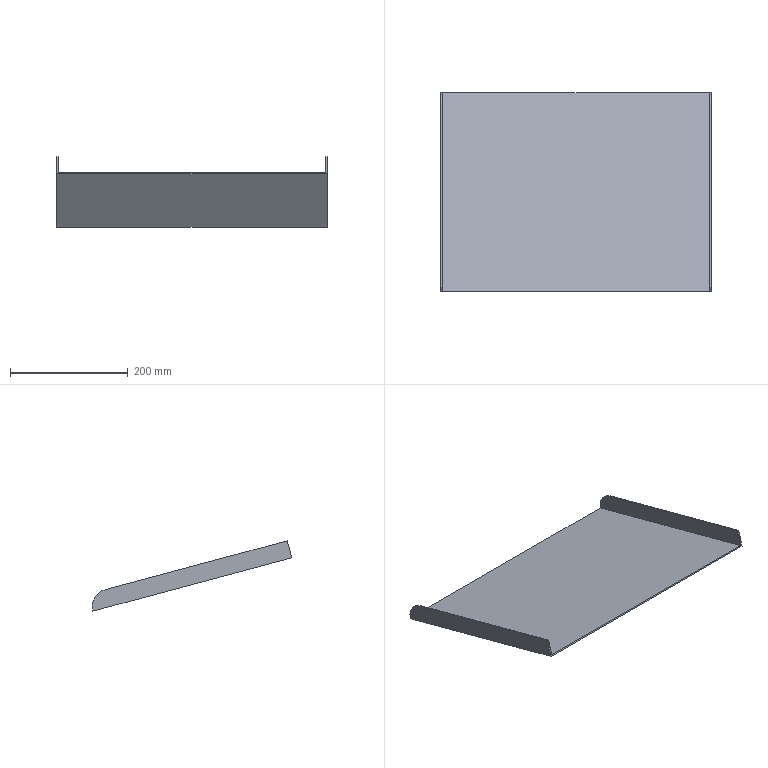Part | NX | features solid 2 | 1 solid | 12 faces | box 459.123 x 339.096 x 119.564 mm | volume 359814 mm3 | plane 10 | cylinder 2 | commonest cylinder face diameters 60 x2
STEP:
#1=CARTESIAN_POINT('',(-416.493,1130.616,-556.061));
#2=VERTEX_POINT('',#1);
#3=CARTESIAN_POINT('',(-414.493,1130.616,-556.061));
#4=VERTEX_POINT('',#3);
#5=CARTESIAN_POINT('',(-426.493,1130.616,-556.061));
#6=DIRECTION('',(-1.,0.,0.));
#7=VECTOR('',#6,1000.);
#8=LINE('',#5,#7);
#9=EDGE_CURVE('',#2,#4,#8,.F.);
#10=ORIENTED_EDGE('',*,*,#9,.T.);
#11=CARTESIAN_POINT('',(-414.493,792.607,-465.492));
#12=VERTEX_POINT('',#11);
#13=CARTESIAN_POINT('',(-414.493,966.473,-512.079));
#14=DIRECTION('',(0.,-0.9659,0.2588));
#15=VECTOR('',#14,1000.);
#16=LINE('',#13,#15);
#17=EDGE_CURVE('',#4,#12,#16,.T.);
#18=ORIENTED_EDGE('',*,*,#17,.T.);
#19=CARTESIAN_POINT('',(40.63,792.607,-465.492));
#20=VERTEX_POINT('',#19);
#21=CARTESIAN_POINT('',(40.63,792.607,-465.492));
#22=DIRECTION('',(-1.,0.,0.));
#23=VECTOR('',#22,1000.);
#24=LINE('',#21,#23);
#25=EDGE_CURVE('',#20,#12,#24,.T.);
#26=ORIENTED_EDGE('',*,*,#25,.F.);
#27=CARTESIAN_POINT('',(40.63,1130.616,-556.061));
#28=VERTEX_POINT('',#27);
#29=CARTESIAN_POINT('',(40.63,966.473,-512.079));
#30=DIRECTION('',(0.,-0.9659,0.2588));
#31=VECTOR('',#30,1000.);
#32=LINE('',#29,#31);
#33=EDGE_CURVE('',#28,#20,#32,.T.);
#34=ORIENTED_EDGE('',*,*,#33,.F.);
#35=CARTESIAN_POINT('',(42.63,1130.616,-556.061));
#36=VERTEX_POINT('',#35);
#37=CARTESIAN_POINT('',(52.63,1130.616,-556.061));
#38=DIRECTION('',(1.,0.,0.));
#39=VECTOR('',#38,1000.);
#40=LINE('',#37,#39);
#41=EDGE_CURVE('',#28,#36,#40,.T.);
#42=ORIENTED_EDGE('',*,*,#41,.T.);
#43=CARTESIAN_POINT('',(42.63,1130.681,-556.078));
#44=VERTEX_POINT('',#43);
#45=CARTESIAN_POINT('',(42.63,966.473,-512.079));
#46=DIRECTION('',(0.,-0.9659,0.2588));
#47=VECTOR('',#46,1000.);
#48=LINE('',#45,#47);
#49=EDGE_CURVE('',#36,#44,#48,.F.);
#50=ORIENTED_EDGE('',*,*,#49,.T.);
#51=CARTESIAN_POINT('',(-416.493,1130.681,-556.078));
#52=VERTEX_POINT('',#51);
#53=CARTESIAN_POINT('',(40.63,1130.681,-556.078));
#54=DIRECTION('',(-1.,0.,0.));
#55=VECTOR('',#54,1000.);
#56=LINE('',#53,#55);
#57=EDGE_CURVE('',#44,#52,#56,.T.);
#58=ORIENTED_EDGE('',*,*,#57,.T.);
#59=CARTESIAN_POINT('',(-416.493,966.473,-512.079));
#60=DIRECTION('',(0.,0.9659,-0.2588));
#61=VECTOR('',#60,1000.);
#62=LINE('',#59,#61);
#63=EDGE_CURVE('',#2,#52,#62,.T.);
#64=ORIENTED_EDGE('',*,*,#63,.F.);
#65=EDGE_LOOP('',(#10,#18,#26,#34,#42,#50,#58,#64));
#66=FACE_BOUND('',#65,.T.);
#67=CARTESIAN_POINT('',(40.63,966.473,-512.079));
#68=DIRECTION('',(0.,-0.2588,-0.9659));
#69=DIRECTION('',(-1.,0.,0.));
#70=AXIS2_PLACEMENT_3D('',#67,#68,#69);
#71=PLANE('',#70);
#72=ADVANCED_FACE('',(#66),#71,.F.);
#73=ORIENTED_EDGE('',*,*,#25,.T.);
#74=CARTESIAN_POINT('',(-414.493,799.853,-438.446));
#75=VERTEX_POINT('',#74);
#76=CARTESIAN_POINT('',(-414.493,792.607,-465.492));
#77=DIRECTION('',(0.,0.2588,0.9659));
#78=VECTOR('',#77,1000.);
#79=LINE('',#76,#78);
#80=EDGE_CURVE('',#12,#75,#79,.T.);
#81=ORIENTED_EDGE('',*,*,#80,.T.);
#82=CARTESIAN_POINT('',(-416.493,799.853,-438.446));
#83=VERTEX_POINT('',#82);
#84=CARTESIAN_POINT('',(-426.493,799.853,-438.446));
#85=DIRECTION('',(-1.,0.,0.));
#86=VECTOR('',#85,1000.);
#87=LINE('',#84,#86);
#88=EDGE_CURVE('',#83,#75,#87,.F.);
#89=ORIENTED_EDGE('',*,*,#88,.F.);
#90=CARTESIAN_POINT('',(-416.493,792.089,-467.423));
#91=VERTEX_POINT('',#90);
#92=CARTESIAN_POINT('',(-416.493,792.607,-465.492));
#93=DIRECTION('',(0.,-0.2588,-0.9659));
#94=VECTOR('',#93,1000.);
#95=LINE('',#92,#94);
#96=EDGE_CURVE('',#83,#91,#95,.T.);
#97=ORIENTED_EDGE('',*,*,#96,.T.);
#98=CARTESIAN_POINT('',(42.63,792.089,-467.423));
#99=VERTEX_POINT('',#98);
#100=CARTESIAN_POINT('',(40.63,792.089,-467.423));
#101=DIRECTION('',(-1.,0.,0.));
#102=VECTOR('',#101,1000.);
#103=LINE('',#100,#102);
#104=EDGE_CURVE('',#99,#91,#103,.T.);
#105=ORIENTED_EDGE('',*,*,#104,.F.);
#106=CARTESIAN_POINT('',(42.63,799.853,-438.446));
#107=VERTEX_POINT('',#106);
#108=CARTESIAN_POINT('',(42.63,792.607,-465.492));
#109=DIRECTION('',(0.,0.2588,0.9659));
#110=VECTOR('',#109,1000.);
#111=LINE('',#108,#110);
#112=EDGE_CURVE('',#107,#99,#111,.F.);
#113=ORIENTED_EDGE('',*,*,#112,.F.);
#114=CARTESIAN_POINT('',(40.63,799.853,-438.446));
#115=VERTEX_POINT('',#114);
#116=CARTESIAN_POINT('',(52.63,799.853,-438.446));
#117=DIRECTION('',(-1.,0.,0.));
#118=VECTOR('',#117,1000.);
#119=LINE('',#116,#118);
#120=EDGE_CURVE('',#107,#115,#119,.T.);
#121=ORIENTED_EDGE('',*,*,#120,.T.);
#122=CARTESIAN_POINT('',(40.63,792.607,-465.492));
#123=DIRECTION('',(0.,0.2588,0.9659));
#124=VECTOR('',#123,1000.);
#125=LINE('',#122,#124);
#126=EDGE_CURVE('',#20,#115,#125,.T.);
#127=ORIENTED_EDGE('',*,*,#126,.F.);
#128=EDGE_LOOP('',(#73,#81,#89,#97,#105,#113,#121,#127));
#129=FACE_BOUND('',#128,.T.);
#130=CARTESIAN_POINT('',(40.63,792.607,-465.492));
#131=DIRECTION('',(0.,-0.9659,0.2588));
#132=DIRECTION('',(-1.,0.,0.));
#133=AXIS2_PLACEMENT_3D('',#130,#131,#132);
#134=PLANE('',#133);
#135=ADVANCED_FACE('',(#129),#134,.T.);
#136=CARTESIAN_POINT('',(-416.493,1130.163,-558.01));
#137=VERTEX_POINT('',#136);
#138=CARTESIAN_POINT('',(-416.493,1130.681,-556.078));
#139=DIRECTION('',(0.,0.2588,0.9659));
#140=VECTOR('',#139,1000.);
#141=LINE('',#138,#140);
#142=EDGE_CURVE('',#52,#137,#141,.F.);
#143=ORIENTED_EDGE('',*,*,#142,.T.);
#144=CARTESIAN_POINT('',(-416.493,965.956,-514.011));
#145=DIRECTION('',(0.,0.9659,-0.2588));
#146=VECTOR('',#145,1000.);
#147=LINE('',#144,#146);
#148=EDGE_CURVE('',#91,#137,#147,.T.);
#149=ORIENTED_EDGE('',*,*,#148,.F.);
#150=ORIENTED_EDGE('',*,*,#96,.F.);
#151=CARTESIAN_POINT('',(-416.493,1108.95,-521.268));
#152=VERTEX_POINT('',#151);
#153=CARTESIAN_POINT('',(-416.493,973.72,-485.033));
#154=DIRECTION('',(0.,-0.9659,0.2588));
#155=VECTOR('',#154,1000.);
#156=LINE('',#153,#155);
#157=EDGE_CURVE('',#83,#152,#156,.F.);
#158=ORIENTED_EDGE('',*,*,#157,.T.);
#159=CARTESIAN_POINT('',(-416.493,1101.185,-550.246));
#160=DIRECTION('',(-1.,0.,0.));
#161=DIRECTION('',(0.,0.,1.));
#162=AXIS2_PLACEMENT_3D('',#159,#160,#161);
#163=CIRCLE('',#162,30.);
#164=EDGE_CURVE('',#152,#2,#163,.T.);
#165=ORIENTED_EDGE('',*,*,#164,.T.);
#166=ORIENTED_EDGE('',*,*,#63,.T.);
#167=EDGE_LOOP('',(#143,#149,#150,#158,#165,#166));
#168=FACE_BOUND('',#167,.T.);
#169=CARTESIAN_POINT('',(-416.493,966.473,-512.079));
#170=DIRECTION('',(-1.,0.,0.));
#171=DIRECTION('',(0.,0.9659,-0.2588));
#172=AXIS2_PLACEMENT_3D('',#169,#170,#171);
#173=PLANE('',#172);
#174=ADVANCED_FACE('',(#168),#173,.T.);
#175=ORIENTED_EDGE('',*,*,#142,.F.);
#176=ORIENTED_EDGE('',*,*,#57,.F.);
#177=CARTESIAN_POINT('',(42.63,1130.163,-558.01));
#178=VERTEX_POINT('',#177);
#179=CARTESIAN_POINT('',(42.63,1130.681,-556.078));
#180=DIRECTION('',(0.,-0.2588,-0.9659));
#181=VECTOR('',#180,1000.);
#182=LINE('',#179,#181);
#183=EDGE_CURVE('',#44,#178,#182,.T.);
#184=ORIENTED_EDGE('',*,*,#183,.T.);
#185=CARTESIAN_POINT('',(40.63,1130.163,-558.01));
#186=DIRECTION('',(-1.,0.,0.));
#187=VECTOR('',#186,1000.);
#188=LINE('',#185,#187);
#189=EDGE_CURVE('',#178,#137,#188,.T.);
#190=ORIENTED_EDGE('',*,*,#189,.T.);
#191=EDGE_LOOP('',(#175,#176,#184,#190));
#192=FACE_BOUND('',#191,.T.);
#193=CARTESIAN_POINT('',(40.63,1130.681,-556.078));
#194=DIRECTION('',(0.,-0.9659,0.2588));
#195=DIRECTION('',(-1.,0.,0.));
#196=AXIS2_PLACEMENT_3D('',#193,#194,#195);
#197=PLANE('',#196);
#198=ADVANCED_FACE('',(#192),#197,.F.);
#199=ORIENTED_EDGE('',*,*,#104,.T.);
#200=ORIENTED_EDGE('',*,*,#148,.T.);
#201=ORIENTED_EDGE('',*,*,#189,.F.);
#202=CARTESIAN_POINT('',(42.63,965.956,-514.011));
#203=DIRECTION('',(0.,-0.9659,0.2588));
#204=VECTOR('',#203,1000.);
#205=LINE('',#202,#204);
#206=EDGE_CURVE('',#99,#178,#205,.F.);
#207=ORIENTED_EDGE('',*,*,#206,.F.);
#208=EDGE_LOOP('',(#199,#200,#201,#207));
#209=FACE_BOUND('',#208,.T.);
#210=CARTESIAN_POINT('',(40.63,965.956,-514.011));
#211=DIRECTION('',(0.,-0.2588,-0.9659));
#212=DIRECTION('',(-1.,0.,0.));
#213=AXIS2_PLACEMENT_3D('',#210,#211,#212);
#214=PLANE('',#213);
#215=ADVANCED_FACE('',(#209),#214,.T.);
#216=ORIENTED_EDGE('',*,*,#49,.F.);
#217=CARTESIAN_POINT('',(42.63,1108.95,-521.268));
#218=VERTEX_POINT('',#217);
#219=CARTESIAN_POINT('',(42.63,1101.185,-550.246));
#220=DIRECTION('',(-1.,0.,0.));
#221=DIRECTION('',(0.,0.,1.));
#222=AXIS2_PLACEMENT_3D('',#219,#220,#221);
#223=CIRCLE('',#222,30.);
#224=EDGE_CURVE('',#36,#218,#223,.F.);
#225=ORIENTED_EDGE('',*,*,#224,.T.);
#226=CARTESIAN_POINT('',(42.63,973.72,-485.033));
#227=DIRECTION('',(0.,-0.9659,0.2588));
#228=VECTOR('',#227,1000.);
#229=LINE('',#226,#228);
#230=EDGE_CURVE('',#107,#218,#229,.F.);
#231=ORIENTED_EDGE('',*,*,#230,.F.);
#232=ORIENTED_EDGE('',*,*,#112,.T.);
#233=ORIENTED_EDGE('',*,*,#206,.T.);
#234=ORIENTED_EDGE('',*,*,#183,.F.);
#235=EDGE_LOOP('',(#216,#225,#231,#232,#233,#234));
#236=FACE_BOUND('',#235,.T.);
#237=CARTESIAN_POINT('',(42.63,966.473,-512.079));
#238=DIRECTION('',(-1.,0.,0.));
#239=DIRECTION('',(0.,0.9659,-0.2588));
#240=AXIS2_PLACEMENT_3D('',#237,#238,#239);
#241=PLANE('',#240);
#242=ADVANCED_FACE('',(#236),#241,.F.);
#243=CARTESIAN_POINT('',(40.63,1108.95,-521.268));
#244=VERTEX_POINT('',#243);
#245=CARTESIAN_POINT('',(40.63,1101.185,-550.246));
#246=DIRECTION('',(1.,0.,0.));
#247=DIRECTION('',(0.,0.,-1.));
#248=AXIS2_PLACEMENT_3D('',#245,#246,#247);
#249=CIRCLE('',#248,30.);
#250=EDGE_CURVE('',#244,#28,#249,.F.);
#251=ORIENTED_EDGE('',*,*,#250,.T.);
#252=ORIENTED_EDGE('',*,*,#33,.T.);
#253=ORIENTED_EDGE('',*,*,#126,.T.);
#254=CARTESIAN_POINT('',(40.63,944.742,-477.269));
#255=DIRECTION('',(0.,0.9659,-0.2588));
#256=VECTOR('',#255,1000.);
#257=LINE('',#254,#256);
#258=EDGE_CURVE('',#115,#244,#257,.T.);
#259=ORIENTED_EDGE('',*,*,#258,.T.);
#260=EDGE_LOOP('',(#251,#252,#253,#259));
#261=FACE_BOUND('',#260,.T.);
#262=CARTESIAN_POINT('',(40.63,936.978,-506.246));
#263=DIRECTION('',(1.,0.,0.));
#264=DIRECTION('',(0.,-0.2588,-0.9659));
#265=AXIS2_PLACEMENT_3D('',#262,#263,#264);
#266=PLANE('',#265);
#267=ADVANCED_FACE('',(#261),#266,.F.);
#268=ORIENTED_EDGE('',*,*,#41,.F.);
#269=ORIENTED_EDGE('',*,*,#250,.F.);
#270=CARTESIAN_POINT('',(52.63,1108.95,-521.268));
#271=DIRECTION('',(1.,0.,0.));
#272=VECTOR('',#271,1000.);
#273=LINE('',#270,#272);
#274=EDGE_CURVE('',#218,#244,#273,.F.);
#275=ORIENTED_EDGE('',*,*,#274,.F.);
#276=ORIENTED_EDGE('',*,*,#224,.F.);
#277=EDGE_LOOP('',(#268,#269,#275,#276));
#278=FACE_BOUND('',#277,.T.);
#279=CARTESIAN_POINT('',(52.63,1101.185,-550.246));
#280=DIRECTION('',(1.,0.,0.));
#281=DIRECTION('',(0.,-0.2588,-0.9659));
#282=AXIS2_PLACEMENT_3D('',#279,#280,#281);
#283=CYLINDRICAL_SURFACE('',#282,30.);
#284=ADVANCED_FACE('',(#278),#283,.T.);
#285=ORIENTED_EDGE('',*,*,#230,.T.);
#286=ORIENTED_EDGE('',*,*,#274,.T.);
#287=ORIENTED_EDGE('',*,*,#258,.F.);
#288=ORIENTED_EDGE('',*,*,#120,.F.);
#289=EDGE_LOOP('',(#285,#286,#287,#288));
#290=FACE_BOUND('',#289,.T.);
#291=CARTESIAN_POINT('',(52.63,944.742,-477.269));
#292=DIRECTION('',(0.,-0.2588,-0.9659));
#293=DIRECTION('',(0.,0.9659,-0.2588));
#294=AXIS2_PLACEMENT_3D('',#291,#292,#293);
#295=PLANE('',#294);
#296=ADVANCED_FACE('',(#290),#295,.F.);
#297=ORIENTED_EDGE('',*,*,#17,.F.);
#298=CARTESIAN_POINT('',(-414.493,1108.95,-521.268));
#299=VERTEX_POINT('',#298);
#300=CARTESIAN_POINT('',(-414.493,1101.185,-550.246));
#301=DIRECTION('',(1.,0.,0.));
#302=DIRECTION('',(0.,0.,-1.));
#303=AXIS2_PLACEMENT_3D('',#300,#301,#302);
#304=CIRCLE('',#303,30.);
#305=EDGE_CURVE('',#4,#299,#304,.T.);
#306=ORIENTED_EDGE('',*,*,#305,.T.);
#307=CARTESIAN_POINT('',(-414.493,944.742,-477.269));
#308=DIRECTION('',(0.,-0.9659,0.2588));
#309=VECTOR('',#308,1000.);
#310=LINE('',#307,#309);
#311=EDGE_CURVE('',#75,#299,#310,.F.);
#312=ORIENTED_EDGE('',*,*,#311,.F.);
#313=ORIENTED_EDGE('',*,*,#80,.F.);
#314=EDGE_LOOP('',(#297,#306,#312,#313));
#315=FACE_BOUND('',#314,.T.);
#316=CARTESIAN_POINT('',(-414.493,936.978,-506.246));
#317=DIRECTION('',(1.,0.,0.));
#318=DIRECTION('',(0.,-0.2588,-0.9659));
#319=AXIS2_PLACEMENT_3D('',#316,#317,#318);
#320=PLANE('',#319);
#321=ADVANCED_FACE('',(#315),#320,.T.);
#322=ORIENTED_EDGE('',*,*,#9,.F.);
#323=ORIENTED_EDGE('',*,*,#164,.F.);
#324=CARTESIAN_POINT('',(-426.493,1108.95,-521.268));
#325=DIRECTION('',(1.,0.,0.));
#326=VECTOR('',#325,1000.);
#327=LINE('',#324,#326);
#328=EDGE_CURVE('',#299,#152,#327,.F.);
#329=ORIENTED_EDGE('',*,*,#328,.F.);
#330=ORIENTED_EDGE('',*,*,#305,.F.);
#331=EDGE_LOOP('',(#322,#323,#329,#330));
#332=FACE_BOUND('',#331,.T.);
#333=CARTESIAN_POINT('',(-426.493,1101.185,-550.246));
#334=DIRECTION('',(-1.,0.,0.));
#335=DIRECTION('',(0.,0.2588,0.9659));
#336=AXIS2_PLACEMENT_3D('',#333,#334,#335);
#337=CYLINDRICAL_SURFACE('',#336,30.);
#338=ADVANCED_FACE('',(#332),#337,.T.);
#339=ORIENTED_EDGE('',*,*,#311,.T.);
#340=ORIENTED_EDGE('',*,*,#328,.T.);
#341=ORIENTED_EDGE('',*,*,#157,.F.);
#342=ORIENTED_EDGE('',*,*,#88,.T.);
#343=EDGE_LOOP('',(#339,#340,#341,#342));
#344=FACE_BOUND('',#343,.T.);
#345=CARTESIAN_POINT('',(-426.493,944.742,-477.269));
#346=DIRECTION('',(0.,-0.2588,-0.9659));
#347=DIRECTION('',(0.,0.9659,-0.2588));
#348=AXIS2_PLACEMENT_3D('',#345,#346,#347);
#349=PLANE('',#348);
#350=ADVANCED_FACE('',(#344),#349,.F.);
#351=CLOSED_SHELL('',(#72,#135,#174,#198,#215,#242,#267,#284,#296,#321,#338,#350));
#352=MANIFOLD_SOLID_BREP('',#351);
#353=(LENGTH_UNIT()NAMED_UNIT(*)SI_UNIT(.MILLI.,.METRE.));
#354=UNCERTAINTY_MEASURE_WITH_UNIT(LENGTH_MEASURE(0.00001),#353,'','');
#355=(NAMED_UNIT(*)PLANE_ANGLE_UNIT()SI_UNIT($,.RADIAN.));
#356=(NAMED_UNIT(*)SI_UNIT($,.STERADIAN.)SOLID_ANGLE_UNIT());
#357=(GEOMETRIC_REPRESENTATION_CONTEXT(3)GLOBAL_UNCERTAINTY_ASSIGNED_CONTEXT((#354))GLOBAL_UNIT_ASSIGNED_CONTEXT((#353,#355,#356))REPRESENTATION_CONTEXT('',''));
#358=ADVANCED_BREP_SHAPE_REPRESENTATION('',(#352),#357);